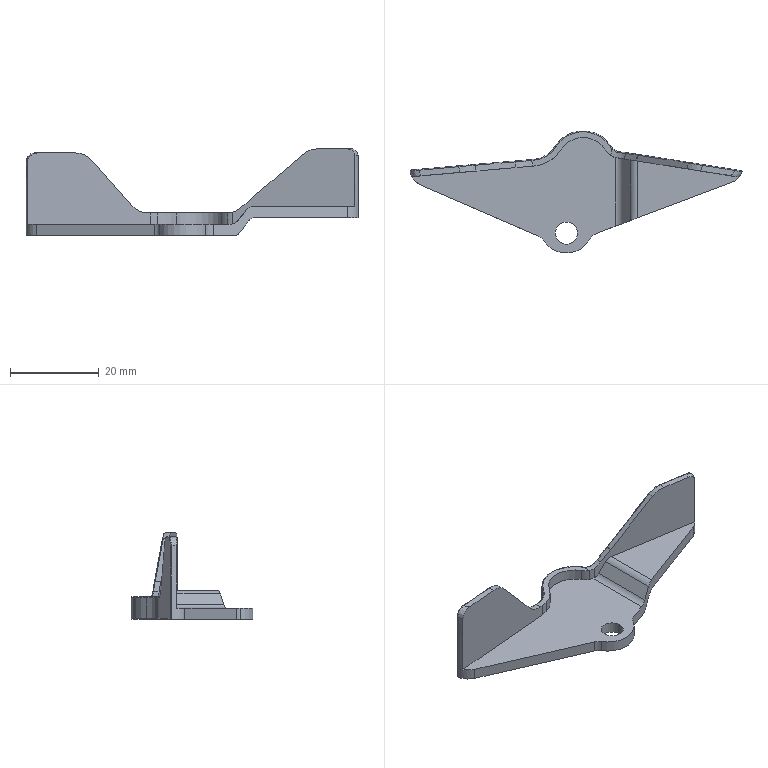Part | STEP file | JDC-75-3 | 1 solid | 89 faces | box 74.72 x 27.5 x 19.44 mm | volume 3290 mm3 | cylinder 41 | plane 24 | torus 11 | spline 11 | other 2 | commonest cylinder face diameters 0.4 x15 4 x4 5 x4 10 x4 8 x3 12 x3